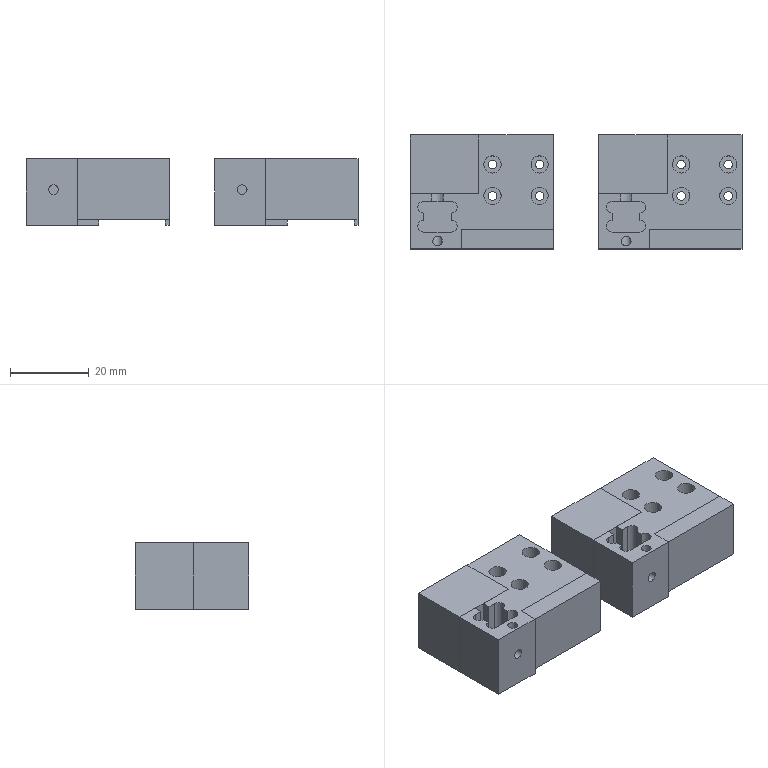NC program | NX | posted with a generic post | part box 84.5 x 29 x 17 mm
Whole program:
N10 G17 G21 G94 G90
(DRILLING_COPY_1 , TOOL : D6A45)
N12 T07 M6
N14 G54
N16 G17 G0 G90 X0.6 Y8.75 B0. C0. S5000 M3
N18 G43 Z30. H7
N20 G94 G81 G98 Z-1.35 F250. R3.
N22 X-2.575 Y14.25
N24 Y3.25
N26 X6.95 Y8.75
N28 G80
N30 G0 X6.95 Y8.75 Z30.
N32 M5
(DRILLING_COPY_COPY_COPY , TOOL : 2.05ZT)
N34 T13 M6
N36 G54
N38 G17 G0 G90 X-2.575 Y3.25 B0. C0. S2000 M3
N40 G43 Z30. H13
N42 G94 G83 G98 Z-5.116 F120. Q2. R3.
N44 Y14.25
N46 X6.95 Y8.75
N48 G80
N50 G0 X6.95 Y8.75 Z30.
N52 M5
(DRILLING_COPY_COPY_COPY_COPY , TOOL : 8.0ZT)
N54 T18 M6
N56 G54
N58 G17 G0 G90 X0.6 Y8.75 B0. C0. S2000 M3
N60 G43 Z30. H18
N62 G94 G83 G98 Z-27.903 F250. Q2. R3.
N64 G80
N66 G0 X0.6 Y8.75 Z30.
N68 M5
(FLOOR_WALL_1_1 , TOOL : D10)
N70 T10 M6
N72 G54
N74 G17 G0 G90 X16.5 Y-23.25 B0. C0. S9500 M3
N76 G43 Z30. H10
N78 Z-11.8
N80 G94 G1 Z-14.8 F1000.
N82 X13.5
N84 X-13.5 F2500.
N86 Y-22.754
N88 X13.5
N90 Y-22.259
N92 X-13.5
N94 Y-21.763
N96 X13.5
N98 Y-21.267
N100 X-13.5
N102 Y-20.771
N104 X13.5
N106 Y-20.276
N108 X-13.5
N110 Y-19.78
N112 X13.5
N114 Y-19.284
N116 X-13.5
N118 Y-18.789
N120 X13.5
N122 Y-18.293
N124 X-13.5
N126 Y-17.797
N128 X13.5
N130 Y-17.301
N132 X-13.5
N134 Y-16.806
N136 X13.5
N138 Y-16.31
N140 X-13.5
N142 Y-15.814
N144 X13.5
N146 Y-15.319
N148 X-13.5
N150 Y-14.823
N152 X13.5
N154 Y-14.327
N156 X-13.5
N158 Y-13.831
N160 X13.5
N162 Y-13.336
N164 X-13.5
N166 Y-12.84
N168 X13.5
N170 Y-12.344
N172 X-13.5
N174 Y-11.849
N176 X13.5
N178 Y-11.353
N180 X-13.5
N182 Y-10.857
N184 X13.5
N186 Y-10.361
N188 X-13.5
N190 Y-9.866
N192 X13.5
N194 Y-9.37
N196 X-13.5
N198 Y-8.874
N200 X13.5
N202 Y-8.379
N204 X-13.5
N206 Y-7.883
N208 X13.5
N210 Y-7.387
N212 X-13.5
N214 Y-6.891
N216 X13.5
N218 Y-6.396
N220 X-13.5
N222 Y-5.9
N224 X13.5
N226 X16.65
N228 Z-11.8
N230 G0 Z30.
(FLOOR_WALL_1_COPY_COPY_COPY_2 , TOOL : D10)
N232 X-14.5 Y-6.753
N234 Z-13.9
N236 G1 Z-14.9 F1000.
N238 X-12.634
N240 G3 X-13.5 Y-6.253 R1.
N242 G1 X13.5 F1500.
N244 Y-10.252
N246 X-13.5
N248 Y-14.25
N250 X13.5
N252 G3 X14.366 Y-13.75 R1.
N254 G1 X14.5 Y-13.518
N256 Z-13.9
N258 G0 Z-8.4
N260 Y-6.482
N262 Z-13.9
N264 G1 Z-14.9 F1000.
N266 X14.366 Y-6.25
N268 G3 X13.5 Y-5.75 R1.
N270 G1 X-13.5 F1500.
N272 G3 X-14.366 Y-6.25 R1.
N274 G1 X-14.5 Y-6.482
N276 Z-13.9
N278 G0 Z30.
N280 M5
(HOLE_MILLING_1 , TOOL : D3)
N282 T03 M6
N284 G54
N286 G17 G0 G90 X0.6 Y-11.25 B0. C0. S9500 M3
N288 G43 Z30. H3
N290 Z-14.4
N292 G94 G3 X0.85 Y-11. R0.25 F1250.
N294 X0.6 Y-10.75 R0.25
N296 X0.6 Y-10.75 Z-14.6 I0. J-0.5
N298 X0.6 Y-10.75 Z-14.8 I0. J-0.5
N300 X0.6 Y-10.75 Z-15. I0. J-0.5
N302 X0.6 Y-10.75 Z-15.2 I0. J-0.5
N304 X0.6 Y-10.75 Z-15.4 I0. J-0.5
N306 X0.6 Y-10.75 Z-15.6 I0. J-0.5
N308 X0.6 Y-10.75 Z-15.8 I0. J-0.5
N310 X0.6 Y-10.75 Z-16. I0. J-0.5
N312 X0.6 Y-10.75 Z-16.2 I0. J-0.5
N314 X0.6 Y-10.75 Z-16.4 I0. J-0.5
N316 X0.6 Y-10.75 Z-16.6 I0. J-0.5
N318 X0.6 Y-10.75 Z-16.8 I0. J-0.5
N320 X0.6 Y-11.75 Z-16.9 I0. J-0.5
N322 X1.1 Y-11.25 R0.5
N324 X0.6 Y-11.75 R-0.5
N326 X0.85 Y-11.5 R0.25
N328 X0.6 Y-11.25 R0.25
N330 G0 Z30.
(PLANAR_PROFILE , TOOL : D3)
N332 X13.
N334 Z-12.05
N336 G1 Z-15.05
N338 X8.5
N340 X1.923
N342 Z-13.55
N344 G0 Z30.
N346 X13.
N348 Z-12.2
N350 G1 Z-15.2
N352 X8.5
N354 X1.923
N356 Z-13.7
N358 G0 Z30.
N360 X13.
N362 Z-12.35
N364 G1 Z-15.35
N366 X8.5
N368 X1.923
N370 Z-13.85
N372 G0 Z30.
N374 X13.
N376 Z-12.5
N378 G1 Z-15.5
N380 X8.5
N382 X1.923
N384 Z-14.
N386 G0 Z30.
N388 X13.
N390 Z-12.65
N392 G1 Z-15.65
N394 X8.5
N396 X1.923
N398 Z-14.15
N400 G0 Z30.
N402 X13.
N404 Z-12.8
N406 G1 Z-15.8
N408 X8.5
N410 X1.923
N412 Z-14.3
N414 G0 Z30.
N416 X13.
N418 Z-12.95
N420 G1 Z-15.95
N422 X8.5
N424 X1.923
N426 Z-14.45
N428 G0 Z30.
N430 X13.
N432 Z-13.1
N434 G1 Z-16.1
N436 X8.5
N438 X1.923
N440 Z-14.6
N442 G0 Z30.
N444 X13.
N446 Z-13.25
N448 G1 Z-16.25
N450 X8.5
N452 X1.923
N454 Z-14.75
N456 G0 Z30.
N458 X13.
N460 Z-13.4
N462 G1 Z-16.4
N464 X8.5
N466 X1.923
N468 Z-14.9
N470 G0 Z30.
N472 X13.
N474 Z-13.55
N476 G1 Z-16.55
N478 X8.5
N480 X1.923
N482 Z-15.05
N484 G0 Z30.
N486 X13.
N488 Z-13.7
N490 G1 Z-16.7
N492 X8.5
N494 X1.923
N496 Z-15.2
N498 G0 Z30.
N500 X13.
N502 Z-13.85
N504 G1 Z-16.85
N506 X8.5
N508 X1.923
N510 Z-15.35
N512 G0 Z30.
N514 X13.
N516 Z-13.9
N518 G1 Z-16.9
N520 X8.5
N522 X1.923
N524 Z-15.4
N526 G0 Z30.
N528 M5
(PLANAR_MILL_COPY_2_COPY_COPY , TOOL : D6A45)
N530 T07 M6
N532 G54
N534 G17 G0 G90 X10.932 Y-4.772 B0. C0. S9500 M3
N536 G43 Z30. H7
N538 Z-12.9
N540 G94 G1 Z-15.9 F1250.
N542 X10.232 Y-4.281
N544 G3 X9.4 Y-4.132 R1.
N546 G1 Y-9.65
N548 G2 X8.4 Y-10.65 R1.
N550 G1 X1.96
N552 G2 X1.312 Y-10.412 R1.
N554 G3 X1.312 Y-12.088 R-1.1
N556 G2 X1.96 Y-11.85 R1.
N558 G1 X8.4
N560 G2 X9.4 Y-12.85 R1.
N562 G1 Y-18.15
N564 G2 X8.4 Y-19.15 R1.
N566 G1 X-8.4
N568 G2 X-9.4 Y-18.15 R1.
N570 G1 Y-4.132
N572 G3 X-10.232 Y-4.281 R1.
N574 G1 X-10.932 Y-4.772
N576 Z-12.9
N578 G0 Z30.
N580 M5
N582 M2